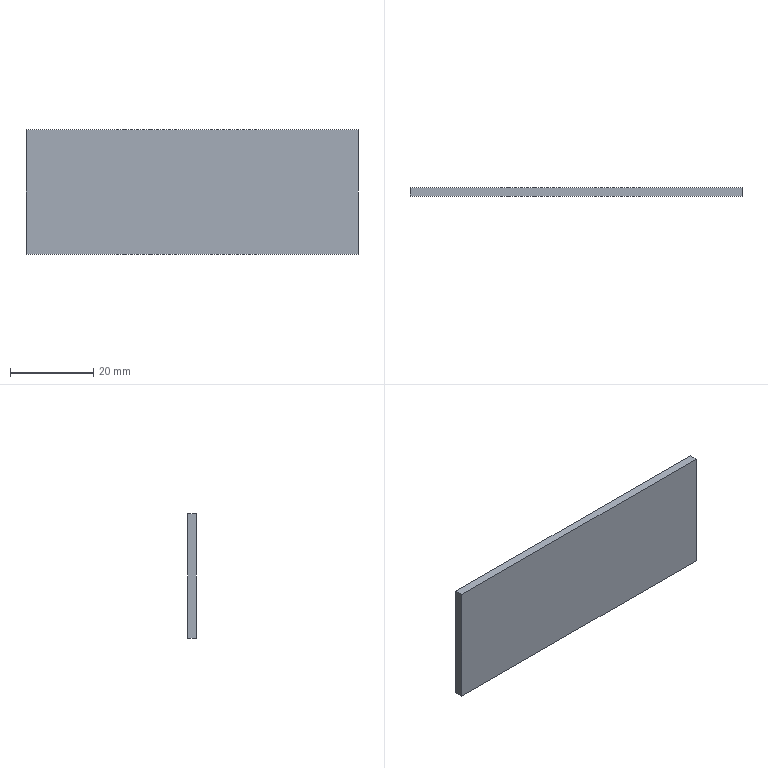Part | STEP file | MYT-A01-P22 | 1 solid | 6 faces | box 80 x 2 x 30 mm | volume 4800 mm3 | plane 6
STEP:
#1=CARTESIAN_POINT('',(0.,-2.,-15.));
#2=VERTEX_POINT('',#1);
#3=CARTESIAN_POINT('',(80.,-2.,-15.));
#4=VERTEX_POINT('',#3);
#5=CARTESIAN_POINT('',(0.,-2.,-15.));
#6=DIRECTION('',(1.,0.,0.));
#7=VECTOR('',#6,1000.);
#8=LINE('',#5,#7);
#9=EDGE_CURVE('',#2,#4,#8,.T.);
#10=ORIENTED_EDGE('',*,*,#9,.T.);
#11=CARTESIAN_POINT('',(80.,-2.,15.));
#12=VERTEX_POINT('',#11);
#13=CARTESIAN_POINT('',(80.,-2.,15.));
#14=DIRECTION('',(0.,0.,-1.));
#15=VECTOR('',#14,1000.);
#16=LINE('',#13,#15);
#17=EDGE_CURVE('',#12,#4,#16,.T.);
#18=ORIENTED_EDGE('',*,*,#17,.F.);
#19=CARTESIAN_POINT('',(0.,-2.,15.));
#20=VERTEX_POINT('',#19);
#21=CARTESIAN_POINT('',(0.,-2.,15.));
#22=DIRECTION('',(1.,0.,0.));
#23=VECTOR('',#22,1000.);
#24=LINE('',#21,#23);
#25=EDGE_CURVE('',#20,#12,#24,.T.);
#26=ORIENTED_EDGE('',*,*,#25,.F.);
#27=CARTESIAN_POINT('',(0.,-2.,15.));
#28=DIRECTION('',(0.,0.,-1.));
#29=VECTOR('',#28,1000.);
#30=LINE('',#27,#29);
#31=EDGE_CURVE('',#20,#2,#30,.T.);
#32=ORIENTED_EDGE('',*,*,#31,.T.);
#33=EDGE_LOOP('',(#10,#18,#26,#32));
#34=FACE_OUTER_BOUND('',#33,.T.);
#35=CARTESIAN_POINT('',(0.,-2.,15.));
#36=DIRECTION('',(0.,1.,0.));
#37=DIRECTION('',(0.,0.,1.));
#38=AXIS2_PLACEMENT_3D('',#35,#36,#37);
#39=PLANE('',#38);
#40=ADVANCED_FACE('',(#34),#39,.F.);
#41=CARTESIAN_POINT('',(80.,0.,-15.));
#42=VERTEX_POINT('',#41);
#43=CARTESIAN_POINT('',(80.,0.,-15.));
#44=DIRECTION('',(0.,-1.,0.));
#45=VECTOR('',#44,1000.);
#46=LINE('',#43,#45);
#47=EDGE_CURVE('',#42,#4,#46,.T.);
#48=ORIENTED_EDGE('',*,*,#47,.F.);
#49=CARTESIAN_POINT('',(80.,0.,15.));
#50=VERTEX_POINT('',#49);
#51=CARTESIAN_POINT('',(80.,0.,15.));
#52=DIRECTION('',(0.,0.,-1.));
#53=VECTOR('',#52,1000.);
#54=LINE('',#51,#53);
#55=EDGE_CURVE('',#50,#42,#54,.T.);
#56=ORIENTED_EDGE('',*,*,#55,.F.);
#57=CARTESIAN_POINT('',(80.,0.,15.));
#58=DIRECTION('',(0.,-1.,0.));
#59=VECTOR('',#58,1000.);
#60=LINE('',#57,#59);
#61=EDGE_CURVE('',#50,#12,#60,.T.);
#62=ORIENTED_EDGE('',*,*,#61,.T.);
#63=ORIENTED_EDGE('',*,*,#17,.T.);
#64=EDGE_LOOP('',(#48,#56,#62,#63));
#65=FACE_OUTER_BOUND('',#64,.T.);
#66=CARTESIAN_POINT('',(80.,0.,15.));
#67=DIRECTION('',(1.,0.,0.));
#68=DIRECTION('',(0.,0.,-1.));
#69=AXIS2_PLACEMENT_3D('',#66,#67,#68);
#70=PLANE('',#69);
#71=ADVANCED_FACE('',(#65),#70,.T.);
#72=CARTESIAN_POINT('',(0.,0.,-15.));
#73=VERTEX_POINT('',#72);
#74=CARTESIAN_POINT('',(0.,0.,-15.));
#75=DIRECTION('',(1.,0.,0.));
#76=VECTOR('',#75,1000.);
#77=LINE('',#74,#76);
#78=EDGE_CURVE('',#73,#42,#77,.T.);
#79=ORIENTED_EDGE('',*,*,#78,.F.);
#80=CARTESIAN_POINT('',(0.,0.,15.));
#81=VERTEX_POINT('',#80);
#82=CARTESIAN_POINT('',(0.,0.,15.));
#83=DIRECTION('',(0.,0.,-1.));
#84=VECTOR('',#83,1000.);
#85=LINE('',#82,#84);
#86=EDGE_CURVE('',#81,#73,#85,.T.);
#87=ORIENTED_EDGE('',*,*,#86,.F.);
#88=CARTESIAN_POINT('',(0.,0.,15.));
#89=DIRECTION('',(1.,0.,0.));
#90=VECTOR('',#89,1000.);
#91=LINE('',#88,#90);
#92=EDGE_CURVE('',#81,#50,#91,.T.);
#93=ORIENTED_EDGE('',*,*,#92,.T.);
#94=ORIENTED_EDGE('',*,*,#55,.T.);
#95=EDGE_LOOP('',(#79,#87,#93,#94));
#96=FACE_OUTER_BOUND('',#95,.T.);
#97=CARTESIAN_POINT('',(0.,0.,15.));
#98=DIRECTION('',(0.,1.,0.));
#99=DIRECTION('',(0.,0.,1.));
#100=AXIS2_PLACEMENT_3D('',#97,#98,#99);
#101=PLANE('',#100);
#102=ADVANCED_FACE('',(#96),#101,.T.);
#103=CARTESIAN_POINT('',(0.,-2.,-15.));
#104=DIRECTION('',(0.,1.,0.));
#105=VECTOR('',#104,1000.);
#106=LINE('',#103,#105);
#107=EDGE_CURVE('',#2,#73,#106,.T.);
#108=ORIENTED_EDGE('',*,*,#107,.F.);
#109=ORIENTED_EDGE('',*,*,#31,.F.);
#110=CARTESIAN_POINT('',(0.,-2.,15.));
#111=DIRECTION('',(0.,1.,0.));
#112=VECTOR('',#111,1000.);
#113=LINE('',#110,#112);
#114=EDGE_CURVE('',#20,#81,#113,.T.);
#115=ORIENTED_EDGE('',*,*,#114,.T.);
#116=ORIENTED_EDGE('',*,*,#86,.T.);
#117=EDGE_LOOP('',(#108,#109,#115,#116));
#118=FACE_OUTER_BOUND('',#117,.T.);
#119=CARTESIAN_POINT('',(0.,-2.,15.));
#120=DIRECTION('',(-1.,0.,0.));
#121=DIRECTION('',(0.,0.,1.));
#122=AXIS2_PLACEMENT_3D('',#119,#120,#121);
#123=PLANE('',#122);
#124=ADVANCED_FACE('',(#118),#123,.T.);
#125=ORIENTED_EDGE('',*,*,#25,.T.);
#126=ORIENTED_EDGE('',*,*,#61,.F.);
#127=ORIENTED_EDGE('',*,*,#92,.F.);
#128=ORIENTED_EDGE('',*,*,#114,.F.);
#129=EDGE_LOOP('',(#125,#126,#127,#128));
#130=FACE_OUTER_BOUND('',#129,.T.);
#131=CARTESIAN_POINT('',(0.,0.,15.));
#132=DIRECTION('',(0.,0.,-1.));
#133=DIRECTION('',(-1.,0.,0.));
#134=AXIS2_PLACEMENT_3D('',#131,#132,#133);
#135=PLANE('',#134);
#136=ADVANCED_FACE('',(#130),#135,.F.);
#137=ORIENTED_EDGE('',*,*,#9,.F.);
#138=ORIENTED_EDGE('',*,*,#107,.T.);
#139=ORIENTED_EDGE('',*,*,#78,.T.);
#140=ORIENTED_EDGE('',*,*,#47,.T.);
#141=EDGE_LOOP('',(#137,#138,#139,#140));
#142=FACE_OUTER_BOUND('',#141,.T.);
#143=CARTESIAN_POINT('',(0.,0.,-15.));
#144=DIRECTION('',(0.,0.,-1.));
#145=DIRECTION('',(-1.,0.,0.));
#146=AXIS2_PLACEMENT_3D('',#143,#144,#145);
#147=PLANE('',#146);
#148=ADVANCED_FACE('',(#142),#147,.T.);
#149=CLOSED_SHELL('',(#40,#71,#102,#124,#136,#148));
#150=MANIFOLD_SOLID_BREP('',#149);
#151=CARTESIAN_POINT('',(0.,0.,0.));
#152=DIRECTION('',(0.,0.,1.));
#153=DIRECTION('',(1.,0.,0.));
#154=AXIS2_PLACEMENT_3D('',#151,#152,#153);
#155=(LENGTH_UNIT()NAMED_UNIT(*)SI_UNIT(.MILLI.,.METRE.));
#156=UNCERTAINTY_MEASURE_WITH_UNIT(LENGTH_MEASURE(0.00001),#155,'','');
#157=(NAMED_UNIT(*)PLANE_ANGLE_UNIT()SI_UNIT($,.RADIAN.));
#158=(NAMED_UNIT(*)SI_UNIT($,.STERADIAN.)SOLID_ANGLE_UNIT());
#159=(GEOMETRIC_REPRESENTATION_CONTEXT(3)GLOBAL_UNCERTAINTY_ASSIGNED_CONTEXT((#156))GLOBAL_UNIT_ASSIGNED_CONTEXT((#155,#157,#158))REPRESENTATION_CONTEXT('',''));
#160=ADVANCED_BREP_SHAPE_REPRESENTATION('',(#150,#154),#159);